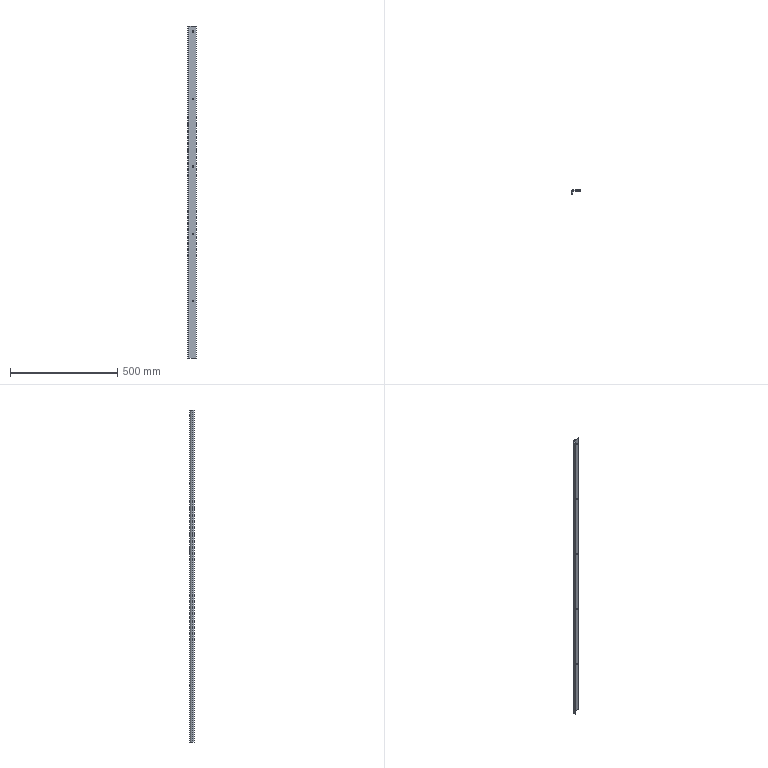Part | SolidWorks | features FlatPattern 1, HoleWzd 1, LPattern 1, SMBaseFlange 1, SheetMetal 1 | 1 solid | 24 faces | box 40 x 19 x 1550 mm | volume 354622 mm3 | cylinder 12 | plane 12 | commonest cylinder face diameters 6.8 x10 12 x1 21 x1
STEP:
#1=CARTESIAN_POINT('',(25.,-4.5,1206.6));
#2=VERTEX_POINT('',#1);
#3=CARTESIAN_POINT('',(25.,-4.5,1213.4));
#4=VERTEX_POINT('',#3);
#5=CARTESIAN_POINT('',(25.,-4.5,1210.));
#6=DIRECTION('',(0.,1.,0.));
#7=DIRECTION('',(0.,0.,1.));
#8=AXIS2_PLACEMENT_3D('',#5,#6,#7);
#9=CIRCLE('',#8,3.4);
#10=EDGE_CURVE('',#2,#4,#9,.T.);
#11=ORIENTED_EDGE('',*,*,#10,.F.);
#12=CARTESIAN_POINT('',(25.,0.,1206.6));
#13=VERTEX_POINT('',#12);
#14=CARTESIAN_POINT('',(25.,0.,1206.6));
#15=DIRECTION('',(0.,1.,0.));
#16=VECTOR('',#15,1000.);
#17=LINE('',#14,#16);
#18=EDGE_CURVE('',#2,#13,#17,.T.);
#19=ORIENTED_EDGE('',*,*,#18,.T.);
#20=CARTESIAN_POINT('',(25.,0.,1213.4));
#21=VERTEX_POINT('',#20);
#22=CARTESIAN_POINT('',(25.,0.,1210.));
#23=DIRECTION('',(0.,1.,0.));
#24=DIRECTION('',(0.,0.,1.));
#25=AXIS2_PLACEMENT_3D('',#22,#23,#24);
#26=CIRCLE('',#25,3.4);
#27=EDGE_CURVE('',#13,#21,#26,.T.);
#28=ORIENTED_EDGE('',*,*,#27,.T.);
#29=CARTESIAN_POINT('',(25.,0.,1213.4));
#30=DIRECTION('',(0.,1.,0.));
#31=VECTOR('',#30,1000.);
#32=LINE('',#29,#31);
#33=EDGE_CURVE('',#4,#21,#32,.T.);
#34=ORIENTED_EDGE('',*,*,#33,.F.);
#35=EDGE_LOOP('',(#11,#19,#28,#34));
#36=FACE_OUTER_BOUND('',#35,.T.);
#37=CARTESIAN_POINT('',(25.,0.,1210.));
#38=DIRECTION('',(0.,1.,0.));
#39=DIRECTION('',(0.,0.,1.));
#40=AXIS2_PLACEMENT_3D('',#37,#38,#39);
#41=CYLINDRICAL_SURFACE('',#40,3.4);
#42=ADVANCED_FACE('',(#36),#41,.F.);
#43=CARTESIAN_POINT('',(25.,-4.5,1521.6));
#44=VERTEX_POINT('',#43);
#45=CARTESIAN_POINT('',(25.,-4.5,1528.4));
#46=VERTEX_POINT('',#45);
#47=CARTESIAN_POINT('',(25.,-4.5,1525.));
#48=DIRECTION('',(0.,1.,0.));
#49=DIRECTION('',(0.,0.,1.));
#50=AXIS2_PLACEMENT_3D('',#47,#48,#49);
#51=CIRCLE('',#50,3.4);
#52=EDGE_CURVE('',#44,#46,#51,.T.);
#53=ORIENTED_EDGE('',*,*,#52,.F.);
#54=CARTESIAN_POINT('',(25.,0.,1521.6));
#55=VERTEX_POINT('',#54);
#56=CARTESIAN_POINT('',(25.,0.,1521.6));
#57=DIRECTION('',(0.,1.,0.));
#58=VECTOR('',#57,1000.);
#59=LINE('',#56,#58);
#60=EDGE_CURVE('',#44,#55,#59,.T.);
#61=ORIENTED_EDGE('',*,*,#60,.T.);
#62=CARTESIAN_POINT('',(25.,0.,1528.4));
#63=VERTEX_POINT('',#62);
#64=CARTESIAN_POINT('',(25.,0.,1525.));
#65=DIRECTION('',(0.,1.,0.));
#66=DIRECTION('',(0.,0.,1.));
#67=AXIS2_PLACEMENT_3D('',#64,#65,#66);
#68=CIRCLE('',#67,3.4);
#69=EDGE_CURVE('',#55,#63,#68,.T.);
#70=ORIENTED_EDGE('',*,*,#69,.T.);
#71=CARTESIAN_POINT('',(25.,0.,1528.4));
#72=DIRECTION('',(0.,1.,0.));
#73=VECTOR('',#72,1000.);
#74=LINE('',#71,#73);
#75=EDGE_CURVE('',#46,#63,#74,.T.);
#76=ORIENTED_EDGE('',*,*,#75,.F.);
#77=EDGE_LOOP('',(#53,#61,#70,#76));
#78=FACE_OUTER_BOUND('',#77,.T.);
#79=CARTESIAN_POINT('',(25.,0.,1525.));
#80=DIRECTION('',(0.,1.,0.));
#81=DIRECTION('',(0.,0.,1.));
#82=AXIS2_PLACEMENT_3D('',#79,#80,#81);
#83=CYLINDRICAL_SURFACE('',#82,3.4);
#84=ADVANCED_FACE('',(#78),#83,.F.);
#85=CARTESIAN_POINT('',(25.,-4.5,891.6));
#86=VERTEX_POINT('',#85);
#87=CARTESIAN_POINT('',(25.,-4.5,898.4));
#88=VERTEX_POINT('',#87);
#89=CARTESIAN_POINT('',(25.,-4.5,895.));
#90=DIRECTION('',(0.,1.,0.));
#91=DIRECTION('',(0.,0.,1.));
#92=AXIS2_PLACEMENT_3D('',#89,#90,#91);
#93=CIRCLE('',#92,3.4);
#94=EDGE_CURVE('',#86,#88,#93,.T.);
#95=ORIENTED_EDGE('',*,*,#94,.F.);
#96=CARTESIAN_POINT('',(25.,0.,891.6));
#97=VERTEX_POINT('',#96);
#98=CARTESIAN_POINT('',(25.,0.,891.6));
#99=DIRECTION('',(0.,1.,0.));
#100=VECTOR('',#99,1000.);
#101=LINE('',#98,#100);
#102=EDGE_CURVE('',#86,#97,#101,.T.);
#103=ORIENTED_EDGE('',*,*,#102,.T.);
#104=CARTESIAN_POINT('',(25.,0.,898.4));
#105=VERTEX_POINT('',#104);
#106=CARTESIAN_POINT('',(25.,0.,895.));
#107=DIRECTION('',(0.,1.,0.));
#108=DIRECTION('',(0.,0.,1.));
#109=AXIS2_PLACEMENT_3D('',#106,#107,#108);
#110=CIRCLE('',#109,3.4);
#111=EDGE_CURVE('',#97,#105,#110,.T.);
#112=ORIENTED_EDGE('',*,*,#111,.T.);
#113=CARTESIAN_POINT('',(25.,0.,898.4));
#114=DIRECTION('',(0.,1.,0.));
#115=VECTOR('',#114,1000.);
#116=LINE('',#113,#115);
#117=EDGE_CURVE('',#88,#105,#116,.T.);
#118=ORIENTED_EDGE('',*,*,#117,.F.);
#119=EDGE_LOOP('',(#95,#103,#112,#118));
#120=FACE_OUTER_BOUND('',#119,.T.);
#121=CARTESIAN_POINT('',(25.,0.,895.));
#122=DIRECTION('',(0.,1.,0.));
#123=DIRECTION('',(0.,0.,1.));
#124=AXIS2_PLACEMENT_3D('',#121,#122,#123);
#125=CYLINDRICAL_SURFACE('',#124,3.4);
#126=ADVANCED_FACE('',(#120),#125,.F.);
#127=CARTESIAN_POINT('',(25.,-4.5,576.6));
#128=VERTEX_POINT('',#127);
#129=CARTESIAN_POINT('',(25.,-4.5,583.4));
#130=VERTEX_POINT('',#129);
#131=CARTESIAN_POINT('',(25.,-4.5,580.));
#132=DIRECTION('',(0.,1.,0.));
#133=DIRECTION('',(0.,0.,1.));
#134=AXIS2_PLACEMENT_3D('',#131,#132,#133);
#135=CIRCLE('',#134,3.4);
#136=EDGE_CURVE('',#128,#130,#135,.T.);
#137=ORIENTED_EDGE('',*,*,#136,.F.);
#138=CARTESIAN_POINT('',(25.,0.,576.6));
#139=VERTEX_POINT('',#138);
#140=CARTESIAN_POINT('',(25.,0.,576.6));
#141=DIRECTION('',(0.,1.,0.));
#142=VECTOR('',#141,1000.);
#143=LINE('',#140,#142);
#144=EDGE_CURVE('',#128,#139,#143,.T.);
#145=ORIENTED_EDGE('',*,*,#144,.T.);
#146=CARTESIAN_POINT('',(25.,0.,583.4));
#147=VERTEX_POINT('',#146);
#148=CARTESIAN_POINT('',(25.,0.,580.));
#149=DIRECTION('',(0.,1.,0.));
#150=DIRECTION('',(0.,0.,1.));
#151=AXIS2_PLACEMENT_3D('',#148,#149,#150);
#152=CIRCLE('',#151,3.4);
#153=EDGE_CURVE('',#139,#147,#152,.T.);
#154=ORIENTED_EDGE('',*,*,#153,.T.);
#155=CARTESIAN_POINT('',(25.,0.,583.4));
#156=DIRECTION('',(0.,1.,0.));
#157=VECTOR('',#156,1000.);
#158=LINE('',#155,#157);
#159=EDGE_CURVE('',#130,#147,#158,.T.);
#160=ORIENTED_EDGE('',*,*,#159,.F.);
#161=EDGE_LOOP('',(#137,#145,#154,#160));
#162=FACE_OUTER_BOUND('',#161,.T.);
#163=CARTESIAN_POINT('',(25.,0.,580.));
#164=DIRECTION('',(0.,1.,0.));
#165=DIRECTION('',(0.,0.,1.));
#166=AXIS2_PLACEMENT_3D('',#163,#164,#165);
#167=CYLINDRICAL_SURFACE('',#166,3.4);
#168=ADVANCED_FACE('',(#162),#167,.F.);
#169=CARTESIAN_POINT('',(25.,-4.5,261.6));
#170=VERTEX_POINT('',#169);
#171=CARTESIAN_POINT('',(25.,-4.5,268.4));
#172=VERTEX_POINT('',#171);
#173=CARTESIAN_POINT('',(25.,-4.5,265.));
#174=DIRECTION('',(0.,1.,0.));
#175=DIRECTION('',(0.,0.,1.));
#176=AXIS2_PLACEMENT_3D('',#173,#174,#175);
#177=CIRCLE('',#176,3.4);
#178=EDGE_CURVE('',#170,#172,#177,.T.);
#179=ORIENTED_EDGE('',*,*,#178,.F.);
#180=CARTESIAN_POINT('',(25.,0.,261.6));
#181=VERTEX_POINT('',#180);
#182=CARTESIAN_POINT('',(25.,0.,261.6));
#183=DIRECTION('',(0.,1.,0.));
#184=VECTOR('',#183,1000.);
#185=LINE('',#182,#184);
#186=EDGE_CURVE('',#170,#181,#185,.T.);
#187=ORIENTED_EDGE('',*,*,#186,.T.);
#188=CARTESIAN_POINT('',(25.,0.,268.4));
#189=VERTEX_POINT('',#188);
#190=CARTESIAN_POINT('',(25.,0.,265.));
#191=DIRECTION('',(0.,1.,0.));
#192=DIRECTION('',(0.,0.,1.));
#193=AXIS2_PLACEMENT_3D('',#190,#191,#192);
#194=CIRCLE('',#193,3.4);
#195=EDGE_CURVE('',#181,#189,#194,.T.);
#196=ORIENTED_EDGE('',*,*,#195,.T.);
#197=CARTESIAN_POINT('',(25.,0.,268.4));
#198=DIRECTION('',(0.,1.,0.));
#199=VECTOR('',#198,1000.);
#200=LINE('',#197,#199);
#201=EDGE_CURVE('',#172,#189,#200,.T.);
#202=ORIENTED_EDGE('',*,*,#201,.F.);
#203=EDGE_LOOP('',(#179,#187,#196,#202));
#204=FACE_OUTER_BOUND('',#203,.T.);
#205=CARTESIAN_POINT('',(25.,0.,265.));
#206=DIRECTION('',(0.,1.,0.));
#207=DIRECTION('',(0.,0.,1.));
#208=AXIS2_PLACEMENT_3D('',#205,#206,#207);
#209=CYLINDRICAL_SURFACE('',#208,3.4);
#210=ADVANCED_FACE('',(#204),#209,.F.);
#211=ORIENTED_EDGE('',*,*,#186,.F.);
#212=CARTESIAN_POINT('',(25.,-4.5,265.));
#213=DIRECTION('',(0.,1.,0.));
#214=DIRECTION('',(0.,0.,1.));
#215=AXIS2_PLACEMENT_3D('',#212,#213,#214);
#216=CIRCLE('',#215,3.4);
#217=EDGE_CURVE('',#172,#170,#216,.T.);
#218=ORIENTED_EDGE('',*,*,#217,.F.);
#219=ORIENTED_EDGE('',*,*,#201,.T.);
#220=CARTESIAN_POINT('',(25.,0.,265.));
#221=DIRECTION('',(0.,1.,0.));
#222=DIRECTION('',(0.,0.,1.));
#223=AXIS2_PLACEMENT_3D('',#220,#221,#222);
#224=CIRCLE('',#223,3.4);
#225=EDGE_CURVE('',#189,#181,#224,.T.);
#226=ORIENTED_EDGE('',*,*,#225,.T.);
#227=EDGE_LOOP('',(#211,#218,#219,#226));
#228=FACE_OUTER_BOUND('',#227,.T.);
#229=CARTESIAN_POINT('',(25.,0.,265.));
#230=DIRECTION('',(0.,1.,0.));
#231=DIRECTION('',(0.,0.,1.));
#232=AXIS2_PLACEMENT_3D('',#229,#230,#231);
#233=CYLINDRICAL_SURFACE('',#232,3.4);
#234=ADVANCED_FACE('',(#228),#233,.F.);
#235=ORIENTED_EDGE('',*,*,#144,.F.);
#236=CARTESIAN_POINT('',(25.,-4.5,580.));
#237=DIRECTION('',(0.,1.,0.));
#238=DIRECTION('',(0.,0.,1.));
#239=AXIS2_PLACEMENT_3D('',#236,#237,#238);
#240=CIRCLE('',#239,3.4);
#241=EDGE_CURVE('',#130,#128,#240,.T.);
#242=ORIENTED_EDGE('',*,*,#241,.F.);
#243=ORIENTED_EDGE('',*,*,#159,.T.);
#244=CARTESIAN_POINT('',(25.,0.,580.));
#245=DIRECTION('',(0.,1.,0.));
#246=DIRECTION('',(0.,0.,1.));
#247=AXIS2_PLACEMENT_3D('',#244,#245,#246);
#248=CIRCLE('',#247,3.4);
#249=EDGE_CURVE('',#147,#139,#248,.T.);
#250=ORIENTED_EDGE('',*,*,#249,.T.);
#251=EDGE_LOOP('',(#235,#242,#243,#250));
#252=FACE_OUTER_BOUND('',#251,.T.);
#253=CARTESIAN_POINT('',(25.,0.,580.));
#254=DIRECTION('',(0.,1.,0.));
#255=DIRECTION('',(0.,0.,1.));
#256=AXIS2_PLACEMENT_3D('',#253,#254,#255);
#257=CYLINDRICAL_SURFACE('',#256,3.4);
#258=ADVANCED_FACE('',(#252),#257,.F.);
#259=ORIENTED_EDGE('',*,*,#102,.F.);
#260=CARTESIAN_POINT('',(25.,-4.5,895.));
#261=DIRECTION('',(0.,1.,0.));
#262=DIRECTION('',(0.,0.,1.));
#263=AXIS2_PLACEMENT_3D('',#260,#261,#262);
#264=CIRCLE('',#263,3.4);
#265=EDGE_CURVE('',#88,#86,#264,.T.);
#266=ORIENTED_EDGE('',*,*,#265,.F.);
#267=ORIENTED_EDGE('',*,*,#117,.T.);
#268=CARTESIAN_POINT('',(25.,0.,895.));
#269=DIRECTION('',(0.,1.,0.));
#270=DIRECTION('',(0.,0.,1.));
#271=AXIS2_PLACEMENT_3D('',#268,#269,#270);
#272=CIRCLE('',#271,3.4);
#273=EDGE_CURVE('',#105,#97,#272,.T.);
#274=ORIENTED_EDGE('',*,*,#273,.T.);
#275=EDGE_LOOP('',(#259,#266,#267,#274));
#276=FACE_OUTER_BOUND('',#275,.T.);
#277=CARTESIAN_POINT('',(25.,0.,895.));
#278=DIRECTION('',(0.,1.,0.));
#279=DIRECTION('',(0.,0.,1.));
#280=AXIS2_PLACEMENT_3D('',#277,#278,#279);
#281=CYLINDRICAL_SURFACE('',#280,3.4);
#282=ADVANCED_FACE('',(#276),#281,.F.);
#283=CARTESIAN_POINT('',(10.5,0.,1550.));
#284=VERTEX_POINT('',#283);
#285=CARTESIAN_POINT('',(10.5,-4.5,1550.));
#286=VERTEX_POINT('',#285);
#287=CARTESIAN_POINT('',(10.5,0.,1550.));
#288=DIRECTION('',(0.,-1.,0.));
#289=VECTOR('',#288,1000.);
#290=LINE('',#287,#289);
#291=EDGE_CURVE('',#284,#286,#290,.T.);
#292=ORIENTED_EDGE('',*,*,#291,.F.);
#293=CARTESIAN_POINT('',(0.,-10.5,1550.));
#294=VERTEX_POINT('',#293);
#295=CARTESIAN_POINT('',(10.5,-10.5,1550.));
#296=DIRECTION('',(0.,0.,-1.));
#297=DIRECTION('',(1.,0.,0.));
#298=AXIS2_PLACEMENT_3D('',#295,#296,#297);
#299=CIRCLE('',#298,10.5);
#300=EDGE_CURVE('',#294,#284,#299,.T.);
#301=ORIENTED_EDGE('',*,*,#300,.F.);
#302=CARTESIAN_POINT('',(4.5,-10.5,1550.));
#303=VERTEX_POINT('',#302);
#304=CARTESIAN_POINT('',(4.5,-10.5,1550.));
#305=DIRECTION('',(-1.,0.,0.));
#306=VECTOR('',#305,1000.);
#307=LINE('',#304,#306);
#308=EDGE_CURVE('',#303,#294,#307,.T.);
#309=ORIENTED_EDGE('',*,*,#308,.F.);
#310=CARTESIAN_POINT('',(10.5,-10.5,1550.));
#311=DIRECTION('',(0.,0.,-1.));
#312=DIRECTION('',(1.,0.,0.));
#313=AXIS2_PLACEMENT_3D('',#310,#311,#312);
#314=CIRCLE('',#313,6.);
#315=EDGE_CURVE('',#303,#286,#314,.T.);
#316=ORIENTED_EDGE('',*,*,#315,.T.);
#317=EDGE_LOOP('',(#292,#301,#309,#316));
#318=FACE_OUTER_BOUND('',#317,.T.);
#319=CARTESIAN_POINT('',(10.5,0.,1550.));
#320=DIRECTION('',(0.,0.,1.));
#321=DIRECTION('',(1.,0.,0.));
#322=AXIS2_PLACEMENT_3D('',#319,#320,#321);
#323=PLANE('',#322);
#324=ADVANCED_FACE('',(#318),#323,.T.);
#325=CARTESIAN_POINT('',(40.,0.,1550.));
#326=VERTEX_POINT('',#325);
#327=CARTESIAN_POINT('',(0.,0.,1550.));
#328=DIRECTION('',(1.,0.,0.));
#329=VECTOR('',#328,1000.);
#330=LINE('',#327,#329);
#331=EDGE_CURVE('',#284,#326,#330,.T.);
#332=ORIENTED_EDGE('',*,*,#331,.F.);
#333=ORIENTED_EDGE('',*,*,#291,.T.);
#334=CARTESIAN_POINT('',(40.,-4.5,1550.));
#335=VERTEX_POINT('',#334);
#336=CARTESIAN_POINT('',(0.,-4.5,1550.));
#337=DIRECTION('',(1.,0.,0.));
#338=VECTOR('',#337,1000.);
#339=LINE('',#336,#338);
#340=EDGE_CURVE('',#286,#335,#339,.T.);
#341=ORIENTED_EDGE('',*,*,#340,.T.);
#342=CARTESIAN_POINT('',(40.,0.,1550.));
#343=DIRECTION('',(0.,-1.,0.));
#344=VECTOR('',#343,1000.);
#345=LINE('',#342,#344);
#346=EDGE_CURVE('',#326,#335,#345,.T.);
#347=ORIENTED_EDGE('',*,*,#346,.F.);
#348=EDGE_LOOP('',(#332,#333,#341,#347));
#349=FACE_OUTER_BOUND('',#348,.T.);
#350=CARTESIAN_POINT('',(4.5,-10.5,1550.));
#351=DIRECTION('',(0.,0.,1.));
#352=DIRECTION('',(1.,0.,0.));
#353=AXIS2_PLACEMENT_3D('',#350,#351,#352);
#354=PLANE('',#353);
#355=ADVANCED_FACE('',(#349),#354,.T.);
#356=CARTESIAN_POINT('',(0.,-10.5,0.));
#357=VERTEX_POINT('',#356);
#358=CARTESIAN_POINT('',(4.5,-10.5,0.));
#359=VERTEX_POINT('',#358);
#360=CARTESIAN_POINT('',(0.,-10.5,0.));
#361=DIRECTION('',(1.,0.,0.));
#362=VECTOR('',#361,1000.);
#363=LINE('',#360,#362);
#364=EDGE_CURVE('',#357,#359,#363,.T.);
#365=ORIENTED_EDGE('',*,*,#364,.F.);
#366=CARTESIAN_POINT('',(10.5,0.,0.));
#367=VERTEX_POINT('',#366);
#368=CARTESIAN_POINT('',(10.5,-10.5,0.));
#369=DIRECTION('',(0.,0.,-1.));
#370=DIRECTION('',(1.,0.,0.));
#371=AXIS2_PLACEMENT_3D('',#368,#369,#370);
#372=CIRCLE('',#371,10.5);
#373=EDGE_CURVE('',#357,#367,#372,.T.);
#374=ORIENTED_EDGE('',*,*,#373,.T.);
#375=CARTESIAN_POINT('',(10.5,-4.5,0.));
#376=VERTEX_POINT('',#375);
#377=CARTESIAN_POINT('',(10.5,-4.5,0.));
#378=DIRECTION('',(0.,1.,0.));
#379=VECTOR('',#378,1000.);
#380=LINE('',#377,#379);
#381=EDGE_CURVE('',#376,#367,#380,.T.);
#382=ORIENTED_EDGE('',*,*,#381,.F.);
#383=CARTESIAN_POINT('',(10.5,-10.5,0.));
#384=DIRECTION('',(0.,0.,-1.));
#385=DIRECTION('',(1.,0.,0.));
#386=AXIS2_PLACEMENT_3D('',#383,#384,#385);
#387=CIRCLE('',#386,6.);
#388=EDGE_CURVE('',#359,#376,#387,.T.);
#389=ORIENTED_EDGE('',*,*,#388,.F.);
#390=EDGE_LOOP('',(#365,#374,#382,#389));
#391=FACE_OUTER_BOUND('',#390,.T.);
#392=CARTESIAN_POINT('',(0.,-10.5,0.));
#393=DIRECTION('',(0.,0.,-1.));
#394=DIRECTION('',(-1.,0.,0.));
#395=AXIS2_PLACEMENT_3D('',#392,#393,#394);
#396=PLANE('',#395);
#397=ADVANCED_FACE('',(#391),#396,.T.);
#398=CARTESIAN_POINT('',(0.,-19.,0.));
#399=VERTEX_POINT('',#398);
#400=CARTESIAN_POINT('',(0.,0.,0.));
#401=DIRECTION('',(0.,1.,0.));
#402=VECTOR('',#401,1000.);
#403=LINE('',#400,#402);
#404=EDGE_CURVE('',#399,#357,#403,.T.);
#405=ORIENTED_EDGE('',*,*,#404,.T.);
#406=ORIENTED_EDGE('',*,*,#364,.T.);
#407=CARTESIAN_POINT('',(4.5,-19.,0.));
#408=VERTEX_POINT('',#407);
#409=CARTESIAN_POINT('',(4.5,0.,0.));
#410=DIRECTION('',(0.,1.,0.));
#411=VECTOR('',#410,1000.);
#412=LINE('',#409,#411);
#413=EDGE_CURVE('',#408,#359,#412,.T.);
#414=ORIENTED_EDGE('',*,*,#413,.F.);
#415=CARTESIAN_POINT('',(4.5,-19.,0.));
#416=DIRECTION('',(-1.,0.,0.));
#417=VECTOR('',#416,1000.);
#418=LINE('',#415,#417);
#419=EDGE_CURVE('',#408,#399,#418,.T.);
#420=ORIENTED_EDGE('',*,*,#419,.T.);
#421=EDGE_LOOP('',(#405,#406,#414,#420));
#422=FACE_OUTER_BOUND('',#421,.T.);
#423=CARTESIAN_POINT('',(10.5,-4.5,0.));
#424=DIRECTION('',(0.,0.,-1.));
#425=DIRECTION('',(-1.,0.,0.));
#426=AXIS2_PLACEMENT_3D('',#423,#424,#425);
#427=PLANE('',#426);
#428=ADVANCED_FACE('',(#422),#427,.T.);
#429=CARTESIAN_POINT('',(25.,-4.5,1210.));
#430=DIRECTION('',(0.,1.,0.));
#431=DIRECTION('',(0.,0.,1.));
#432=AXIS2_PLACEMENT_3D('',#429,#430,#431);
#433=CIRCLE('',#432,3.4);
#434=EDGE_CURVE('',#4,#2,#433,.T.);
#435=ORIENTED_EDGE('',*,*,#434,.T.);
#436=ORIENTED_EDGE('',*,*,#10,.T.);
#437=EDGE_LOOP('',(#435,#436));
#438=FACE_BOUND('',#437,.T.);
#439=CARTESIAN_POINT('',(25.,-4.5,1525.));
#440=DIRECTION('',(0.,1.,0.));
#441=DIRECTION('',(0.,0.,1.));
#442=AXIS2_PLACEMENT_3D('',#439,#440,#441);
#443=CIRCLE('',#442,3.4);
#444=EDGE_CURVE('',#46,#44,#443,.T.);
#445=ORIENTED_EDGE('',*,*,#444,.T.);
#446=ORIENTED_EDGE('',*,*,#52,.T.);
#447=EDGE_LOOP('',(#445,#446));
#448=FACE_BOUND('',#447,.T.);
#449=CARTESIAN_POINT('',(40.,-4.5,0.));
#450=VERTEX_POINT('',#449);
#451=CARTESIAN_POINT('',(0.,-4.5,0.));
#452=DIRECTION('',(1.,0.,0.));
#453=VECTOR('',#452,1000.);
#454=LINE('',#451,#453);
#455=EDGE_CURVE('',#376,#450,#454,.T.);
#456=ORIENTED_EDGE('',*,*,#455,.T.);
#457=CARTESIAN_POINT('',(40.,-4.5,1550.));
#458=DIRECTION('',(0.,0.,-1.));
#459=VECTOR('',#458,1000.);
#460=LINE('',#457,#459);
#461=EDGE_CURVE('',#335,#450,#460,.T.);
#462=ORIENTED_EDGE('',*,*,#461,.F.);
#463=ORIENTED_EDGE('',*,*,#340,.F.);
#464=CARTESIAN_POINT('',(10.5,-4.5,1550.));
#465=DIRECTION('',(0.,0.,-1.));
#466=VECTOR('',#465,1000.);
#467=LINE('',#464,#466);
#468=EDGE_CURVE('',#286,#376,#467,.T.);
#469=ORIENTED_EDGE('',*,*,#468,.T.);
#470=EDGE_LOOP('',(#456,#462,#463,#469));
#471=FACE_OUTER_BOUND('',#470,.T.);
#472=ORIENTED_EDGE('',*,*,#265,.T.);
#473=ORIENTED_EDGE('',*,*,#94,.T.);
#474=EDGE_LOOP('',(#472,#473));
#475=FACE_BOUND('',#474,.T.);
#476=ORIENTED_EDGE('',*,*,#241,.T.);
#477=ORIENTED_EDGE('',*,*,#136,.T.);
#478=EDGE_LOOP('',(#476,#477));
#479=FACE_BOUND('',#478,.T.);
#480=ORIENTED_EDGE('',*,*,#217,.T.);
#481=ORIENTED_EDGE('',*,*,#178,.T.);
#482=EDGE_LOOP('',(#480,#481));
#483=FACE_BOUND('',#482,.T.);
#484=CARTESIAN_POINT('',(0.,-4.5,1550.));
#485=DIRECTION('',(0.,1.,0.));
#486=DIRECTION('',(0.,0.,1.));
#487=AXIS2_PLACEMENT_3D('',#484,#485,#486);
#488=PLANE('',#487);
#489=ADVANCED_FACE('',(#438,#448,#471,#475,#479,#483),#488,.F.);
#490=CARTESIAN_POINT('',(40.,0.,0.));
#491=VERTEX_POINT('',#490);
#492=CARTESIAN_POINT('',(40.,0.,0.));
#493=DIRECTION('',(0.,-1.,0.));
#494=VECTOR('',#493,1000.);
#495=LINE('',#492,#494);
#496=EDGE_CURVE('',#491,#450,#495,.T.);
#497=ORIENTED_EDGE('',*,*,#496,.F.);
#498=CARTESIAN_POINT('',(40.,0.,1550.));
#499=DIRECTION('',(0.,0.,-1.));
#500=VECTOR('',#499,1000.);
#501=LINE('',#498,#500);
#502=EDGE_CURVE('',#326,#491,#501,.T.);
#503=ORIENTED_EDGE('',*,*,#502,.F.);
#504=ORIENTED_EDGE('',*,*,#346,.T.);
#505=ORIENTED_EDGE('',*,*,#461,.T.);
#506=EDGE_LOOP('',(#497,#503,#504,#505));
#507=FACE_OUTER_BOUND('',#506,.T.);
#508=CARTESIAN_POINT('',(40.,0.,1550.));
#509=DIRECTION('',(1.,0.,0.));
#510=DIRECTION('',(0.,0.,-1.));
#511=AXIS2_PLACEMENT_3D('',#508,#509,#510);
#512=PLANE('',#511);
#513=ADVANCED_FACE('',(#507),#512,.T.);
#514=CARTESIAN_POINT('',(25.,0.,1210.));
#515=DIRECTION('',(0.,1.,0.));
#516=DIRECTION('',(0.,0.,1.));
#517=AXIS2_PLACEMENT_3D('',#514,#515,#516);
#518=CIRCLE('',#517,3.4);
#519=EDGE_CURVE('',#21,#13,#518,.T.);
#520=ORIENTED_EDGE('',*,*,#519,.F.);
#521=ORIENTED_EDGE('',*,*,#27,.F.);
#522=EDGE_LOOP('',(#520,#521));
#523=FACE_BOUND('',#522,.T.);
#524=CARTESIAN_POINT('',(25.,0.,1525.));
#525=DIRECTION('',(0.,1.,0.));
#526=DIRECTION('',(0.,0.,1.));
#527=AXIS2_PLACEMENT_3D('',#524,#525,#526);
#528=CIRCLE('',#527,3.4);
#529=EDGE_CURVE('',#63,#55,#528,.T.);
#530=ORIENTED_EDGE('',*,*,#529,.F.);
#531=ORIENTED_EDGE('',*,*,#69,.F.);
#532=EDGE_LOOP('',(#530,#531));
#533=FACE_BOUND('',#532,.T.);
#534=CARTESIAN_POINT('',(0.,0.,0.));
#535=DIRECTION('',(1.,0.,0.));
#536=VECTOR('',#535,1000.);
#537=LINE('',#534,#536);
#538=EDGE_CURVE('',#367,#491,#537,.T.);
#539=ORIENTED_EDGE('',*,*,#538,.F.);
#540=CARTESIAN_POINT('',(10.5,0.,1550.));
#541=DIRECTION('',(0.,0.,-1.));
#542=VECTOR('',#541,1000.);
#543=LINE('',#540,#542);
#544=EDGE_CURVE('',#284,#367,#543,.T.);
#545=ORIENTED_EDGE('',*,*,#544,.F.);
#546=ORIENTED_EDGE('',*,*,#331,.T.);
#547=ORIENTED_EDGE('',*,*,#502,.T.);
#548=EDGE_LOOP('',(#539,#545,#546,#547));
#549=FACE_OUTER_BOUND('',#548,.T.);
#550=ORIENTED_EDGE('',*,*,#273,.F.);
#551=ORIENTED_EDGE('',*,*,#111,.F.);
#552=EDGE_LOOP('',(#550,#551));
#553=FACE_BOUND('',#552,.T.);
#554=ORIENTED_EDGE('',*,*,#249,.F.);
#555=ORIENTED_EDGE('',*,*,#153,.F.);
#556=EDGE_LOOP('',(#554,#555));
#557=FACE_BOUND('',#556,.T.);
#558=ORIENTED_EDGE('',*,*,#225,.F.);
#559=ORIENTED_EDGE('',*,*,#195,.F.);
#560=EDGE_LOOP('',(#558,#559));
#561=FACE_BOUND('',#560,.T.);
#562=CARTESIAN_POINT('',(0.,0.,1550.));
#563=DIRECTION('',(0.,1.,0.));
#564=DIRECTION('',(0.,0.,1.));
#565=AXIS2_PLACEMENT_3D('',#562,#563,#564);
#566=PLANE('',#565);
#567=ADVANCED_FACE('',(#523,#533,#549,#553,#557,#561),#566,.T.);
#568=ORIENTED_EDGE('',*,*,#373,.F.);
#569=CARTESIAN_POINT('',(0.,-10.5,1550.));
#570=DIRECTION('',(0.,0.,-1.));
#571=VECTOR('',#570,1000.);
#572=LINE('',#569,#571);
#573=EDGE_CURVE('',#294,#357,#572,.T.);
#574=ORIENTED_EDGE('',*,*,#573,.F.);
#575=ORIENTED_EDGE('',*,*,#300,.T.);
#576=ORIENTED_EDGE('',*,*,#544,.T.);
#577=EDGE_LOOP('',(#568,#574,#575,#576));
#578=FACE_OUTER_BOUND('',#577,.T.);
#579=CARTESIAN_POINT('',(10.5,-10.5,1550.));
#580=DIRECTION('',(0.,0.,-1.));
#581=DIRECTION('',(-1.,0.,0.));
#582=AXIS2_PLACEMENT_3D('',#579,#580,#581);
#583=CYLINDRICAL_SURFACE('',#582,10.5);
#584=ADVANCED_FACE('',(#578),#583,.T.);
#585=ORIENTED_EDGE('',*,*,#404,.F.);
#586=CARTESIAN_POINT('',(0.,-19.,1550.));
#587=VERTEX_POINT('',#586);
#588=CARTESIAN_POINT('',(0.,-19.,1550.));
#589=DIRECTION('',(0.,0.,-1.));
#590=VECTOR('',#589,1000.);
#591=LINE('',#588,#590);
#592=EDGE_CURVE('',#587,#399,#591,.T.);
#593=ORIENTED_EDGE('',*,*,#592,.F.);
#594=CARTESIAN_POINT('',(0.,0.,1550.));
#595=DIRECTION('',(0.,1.,0.));
#596=VECTOR('',#595,1000.);
#597=LINE('',#594,#596);
#598=EDGE_CURVE('',#587,#294,#597,.T.);
#599=ORIENTED_EDGE('',*,*,#598,.T.);
#600=ORIENTED_EDGE('',*,*,#573,.T.);
#601=EDGE_LOOP('',(#585,#593,#599,#600));
#602=FACE_OUTER_BOUND('',#601,.T.);
#603=CARTESIAN_POINT('',(0.,0.,1550.));
#604=DIRECTION('',(-1.,0.,0.));
#605=DIRECTION('',(0.,0.,1.));
#606=AXIS2_PLACEMENT_3D('',#603,#604,#605);
#607=PLANE('',#606);
#608=ADVANCED_FACE('',(#602),#607,.T.);
#609=ORIENTED_EDGE('',*,*,#419,.F.);
#610=CARTESIAN_POINT('',(4.5,-19.,1550.));
#611=VERTEX_POINT('',#610);
#612=CARTESIAN_POINT('',(4.5,-19.,1550.));
#613=DIRECTION('',(0.,0.,-1.));
#614=VECTOR('',#613,1000.);
#615=LINE('',#612,#614);
#616=EDGE_CURVE('',#611,#408,#615,.T.);
#617=ORIENTED_EDGE('',*,*,#616,.F.);
#618=CARTESIAN_POINT('',(4.5,-19.,1550.));
#619=DIRECTION('',(-1.,0.,0.));
#620=VECTOR('',#619,1000.);
#621=LINE('',#618,#620);
#622=EDGE_CURVE('',#611,#587,#621,.T.);
#623=ORIENTED_EDGE('',*,*,#622,.T.);
#624=ORIENTED_EDGE('',*,*,#592,.T.);
#625=EDGE_LOOP('',(#609,#617,#623,#624));
#626=FACE_OUTER_BOUND('',#625,.T.);
#627=CARTESIAN_POINT('',(4.5,-19.,1550.));
#628=DIRECTION('',(0.,-1.,0.));
#629=DIRECTION('',(0.,0.,-1.));
#630=AXIS2_PLACEMENT_3D('',#627,#628,#629);
#631=PLANE('',#630);
#632=ADVANCED_FACE('',(#626),#631,.T.);
#633=ORIENTED_EDGE('',*,*,#413,.T.);
#634=CARTESIAN_POINT('',(4.5,-10.5,1550.));
#635=DIRECTION('',(0.,0.,-1.));
#636=VECTOR('',#635,1000.);
#637=LINE('',#634,#636);
#638=EDGE_CURVE('',#303,#359,#637,.T.);
#639=ORIENTED_EDGE('',*,*,#638,.F.);
#640=CARTESIAN_POINT('',(4.5,0.,1550.));
#641=DIRECTION('',(0.,1.,0.));
#642=VECTOR('',#641,1000.);
#643=LINE('',#640,#642);
#644=EDGE_CURVE('',#611,#303,#643,.T.);
#645=ORIENTED_EDGE('',*,*,#644,.F.);
#646=ORIENTED_EDGE('',*,*,#616,.T.);
#647=EDGE_LOOP('',(#633,#639,#645,#646));
#648=FACE_OUTER_BOUND('',#647,.T.);
#649=CARTESIAN_POINT('',(4.5,0.,1550.));
#650=DIRECTION('',(-1.,0.,0.));
#651=DIRECTION('',(0.,0.,1.));
#652=AXIS2_PLACEMENT_3D('',#649,#650,#651);
#653=PLANE('',#652);
#654=ADVANCED_FACE('',(#648),#653,.F.);
#655=ORIENTED_EDGE('',*,*,#388,.T.);
#656=ORIENTED_EDGE('',*,*,#468,.F.);
#657=ORIENTED_EDGE('',*,*,#315,.F.);
#658=ORIENTED_EDGE('',*,*,#638,.T.);
#659=EDGE_LOOP('',(#655,#656,#657,#658));
#660=FACE_OUTER_BOUND('',#659,.T.);
#661=CARTESIAN_POINT('',(10.5,-10.5,1550.));
#662=DIRECTION('',(0.,0.,-1.));
#663=DIRECTION('',(-1.,0.,0.));
#664=AXIS2_PLACEMENT_3D('',#661,#662,#663);
#665=CYLINDRICAL_SURFACE('',#664,6.);
#666=ADVANCED_FACE('',(#660),#665,.F.);
#667=ORIENTED_EDGE('',*,*,#644,.T.);
#668=ORIENTED_EDGE('',*,*,#308,.T.);
#669=ORIENTED_EDGE('',*,*,#598,.F.);
#670=ORIENTED_EDGE('',*,*,#622,.F.);
#671=EDGE_LOOP('',(#667,#668,#669,#670));
#672=FACE_OUTER_BOUND('',#671,.T.);
#673=CARTESIAN_POINT('',(10.5,-10.5,1550.));
#674=DIRECTION('',(0.,0.,1.));
#675=DIRECTION('',(1.,0.,0.));
#676=AXIS2_PLACEMENT_3D('',#673,#674,#675);
#677=PLANE('',#676);
#678=ADVANCED_FACE('',(#672),#677,.T.);
#679=ORIENTED_EDGE('',*,*,#455,.F.);
#680=ORIENTED_EDGE('',*,*,#381,.T.);
#681=ORIENTED_EDGE('',*,*,#538,.T.);
#682=ORIENTED_EDGE('',*,*,#496,.T.);
#683=EDGE_LOOP('',(#679,#680,#681,#682));
#684=FACE_OUTER_BOUND('',#683,.T.);
#685=CARTESIAN_POINT('',(10.5,-10.5,0.));
#686=DIRECTION('',(0.,0.,1.));
#687=DIRECTION('',(1.,0.,0.));
#688=AXIS2_PLACEMENT_3D('',#685,#686,#687);
#689=PLANE('',#688);
#690=ADVANCED_FACE('',(#684),#689,.F.);
#691=ORIENTED_EDGE('',*,*,#60,.F.);
#692=ORIENTED_EDGE('',*,*,#444,.F.);
#693=ORIENTED_EDGE('',*,*,#75,.T.);
#694=ORIENTED_EDGE('',*,*,#529,.T.);
#695=EDGE_LOOP('',(#691,#692,#693,#694));
#696=FACE_OUTER_BOUND('',#695,.T.);
#697=CARTESIAN_POINT('',(25.,0.,1525.));
#698=DIRECTION('',(0.,1.,0.));
#699=DIRECTION('',(0.,0.,1.));
#700=AXIS2_PLACEMENT_3D('',#697,#698,#699);
#701=CYLINDRICAL_SURFACE('',#700,3.4);
#702=ADVANCED_FACE('',(#696),#701,.F.);
#703=ORIENTED_EDGE('',*,*,#18,.F.);
#704=ORIENTED_EDGE('',*,*,#434,.F.);
#705=ORIENTED_EDGE('',*,*,#33,.T.);
#706=ORIENTED_EDGE('',*,*,#519,.T.);
#707=EDGE_LOOP('',(#703,#704,#705,#706));
#708=FACE_OUTER_BOUND('',#707,.T.);
#709=CARTESIAN_POINT('',(25.,0.,1210.));
#710=DIRECTION('',(0.,1.,0.));
#711=DIRECTION('',(0.,0.,1.));
#712=AXIS2_PLACEMENT_3D('',#709,#710,#711);
#713=CYLINDRICAL_SURFACE('',#712,3.4);
#714=ADVANCED_FACE('',(#708),#713,.F.);
#715=CLOSED_SHELL('',(#42,#84,#126,#168,#210,#234,#258,#282,#324,#355,#397,#428,#489,#513,#567,#584,#608,#632,#654,#666,#678,#690,#702,#714));
#716=MANIFOLD_SOLID_BREP('',#715);
#717=CARTESIAN_POINT('',(0.,0.,0.));
#718=DIRECTION('',(0.,0.,1.));
#719=DIRECTION('',(1.,0.,0.));
#720=AXIS2_PLACEMENT_3D('',#717,#718,#719);
#721=(LENGTH_UNIT()NAMED_UNIT(*)SI_UNIT(.MILLI.,.METRE.));
#722=UNCERTAINTY_MEASURE_WITH_UNIT(LENGTH_MEASURE(0.00001),#721,'','');
#723=(NAMED_UNIT(*)PLANE_ANGLE_UNIT()SI_UNIT($,.RADIAN.));
#724=(NAMED_UNIT(*)SI_UNIT($,.STERADIAN.)SOLID_ANGLE_UNIT());
#725=(GEOMETRIC_REPRESENTATION_CONTEXT(3)GLOBAL_UNCERTAINTY_ASSIGNED_CONTEXT((#722))GLOBAL_UNIT_ASSIGNED_CONTEXT((#721,#723,#724))REPRESENTATION_CONTEXT('',''));
#726=ADVANCED_BREP_SHAPE_REPRESENTATION('',(#716,#720),#725);